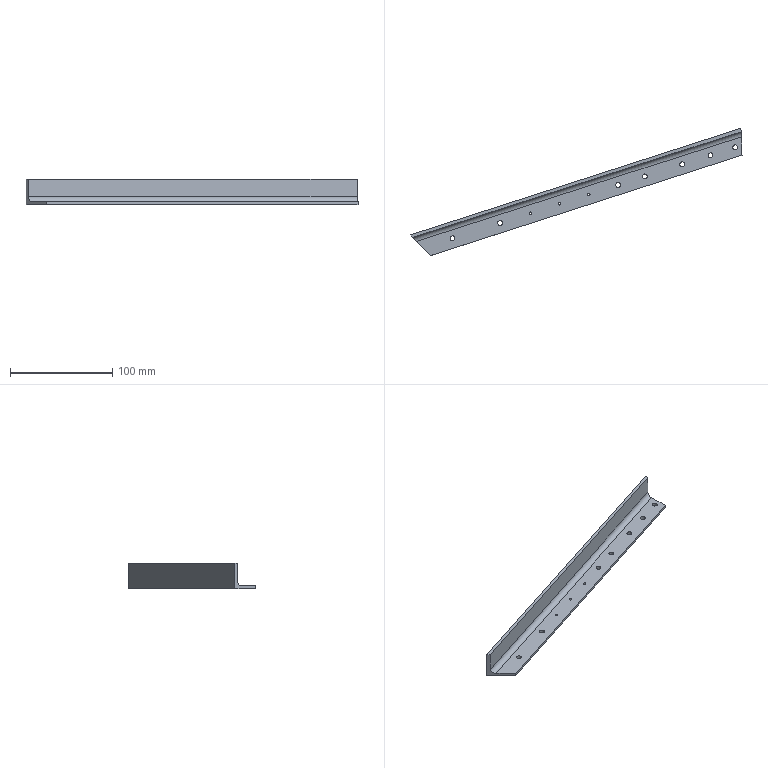Part | NX | features MG0301 nose pivot 24(right) 2 | 1 solid | 19 faces | box 324.725 x 124.459 x 25.4 mm | volume 51732 mm3 | cylinder 11 | plane 8 | commonest cylinder face diameters 4.763 x7 2.4 x3 9.525 x1
STEP:
#1=CARTESIAN_POINT('',(-201.575,-73.399,0.));
#2=VERTEX_POINT('',#1);
#3=CARTESIAN_POINT('',(-202.775,-73.399,0.));
#4=DIRECTION('',(0.,0.,1.));
#5=DIRECTION('',(1.,0.,0.));
#6=AXIS2_PLACEMENT_3D('',#3,#4,#5);
#7=CIRCLE('',#6,1.2);
#8=EDGE_CURVE('',#2,#2,#7,.F.);
#9=ORIENTED_EDGE('',*,*,#8,.F.);
#10=EDGE_LOOP('',(#9));
#11=FACE_BOUND('',#10,.T.);
#12=CARTESIAN_POINT('',(-143.279,-55.017,0.));
#13=VERTEX_POINT('',#12);
#14=CARTESIAN_POINT('',(-145.66,-55.017,0.));
#15=DIRECTION('',(0.,0.,1.));
#16=DIRECTION('',(1.,0.,0.));
#17=AXIS2_PLACEMENT_3D('',#14,#15,#16);
#18=CIRCLE('',#17,2.381);
#19=EDGE_CURVE('',#13,#13,#18,.F.);
#20=ORIENTED_EDGE('',*,*,#19,.F.);
#21=EDGE_LOOP('',(#20));
#22=FACE_BOUND('',#21,.T.);
#23=CARTESIAN_POINT('',(-80.464,-34.801,0.));
#24=VERTEX_POINT('',#23);
#25=CARTESIAN_POINT('',(-82.845,-34.801,0.));
#26=DIRECTION('',(0.,0.,1.));
#27=DIRECTION('',(1.,0.,0.));
#28=AXIS2_PLACEMENT_3D('',#25,#26,#27);
#29=CIRCLE('',#28,2.381);
#30=EDGE_CURVE('',#24,#24,#29,.F.);
#31=ORIENTED_EDGE('',*,*,#30,.F.);
#32=EDGE_LOOP('',(#31));
#33=FACE_BOUND('',#32,.T.);
#34=CARTESIAN_POINT('',(-258.604,-92.134,0.));
#35=VERTEX_POINT('',#34);
#36=CARTESIAN_POINT('',(-260.985,-92.134,0.));
#37=DIRECTION('',(0.,0.,1.));
#38=DIRECTION('',(1.,0.,0.));
#39=AXIS2_PLACEMENT_3D('',#36,#37,#38);
#40=CIRCLE('',#39,2.381);
#41=EDGE_CURVE('',#35,#35,#40,.T.);
#42=ORIENTED_EDGE('',*,*,#41,.T.);
#43=EDGE_LOOP('',(#42));
#44=FACE_BOUND('',#43,.T.);
#45=CARTESIAN_POINT('',(-305.21,-107.134,0.));
#46=VERTEX_POINT('',#45);
#47=CARTESIAN_POINT('',(-307.591,-107.134,0.));
#48=DIRECTION('',(0.,0.,1.));
#49=DIRECTION('',(1.,0.,0.));
#50=AXIS2_PLACEMENT_3D('',#47,#48,#49);
#51=CIRCLE('',#50,2.381);
#52=EDGE_CURVE('',#46,#46,#51,.T.);
#53=ORIENTED_EDGE('',*,*,#52,.T.);
#54=EDGE_LOOP('',(#53));
#55=FACE_BOUND('',#54,.T.);
#56=CARTESIAN_POINT('',(-28.683,-18.135,0.));
#57=VERTEX_POINT('',#56);
#58=CARTESIAN_POINT('',(-31.064,-18.135,0.));
#59=DIRECTION('',(0.,0.,1.));
#60=DIRECTION('',(1.,0.,0.));
#61=AXIS2_PLACEMENT_3D('',#58,#59,#60);
#62=CIRCLE('',#61,2.381);
#63=EDGE_CURVE('',#57,#57,#62,.T.);
#64=ORIENTED_EDGE('',*,*,#63,.T.);
#65=EDGE_LOOP('',(#64));
#66=FACE_BOUND('',#65,.T.);
#67=CARTESIAN_POINT('',(-52.861,-25.917,0.));
#68=VERTEX_POINT('',#67);
#69=CARTESIAN_POINT('',(-55.242,-25.917,0.));
#70=DIRECTION('',(0.,0.,1.));
#71=DIRECTION('',(1.,0.,0.));
#72=AXIS2_PLACEMENT_3D('',#69,#70,#71);
#73=CIRCLE('',#72,2.381);
#74=EDGE_CURVE('',#68,#68,#73,.T.);
#75=ORIENTED_EDGE('',*,*,#74,.T.);
#76=EDGE_LOOP('',(#75));
#77=FACE_BOUND('',#76,.T.);
#78=CARTESIAN_POINT('',(-24.401,-25.997,0.));
#79=VERTEX_POINT('',#78);
#80=CARTESIAN_POINT('',(-329.234,-124.106,0.));
#81=VERTEX_POINT('',#80);
#82=CARTESIAN_POINT('',(-9.84,-21.311,0.));
#83=DIRECTION('',(-0.9519,-0.3064,0.));
#84=VECTOR('',#83,1000.);
#85=LINE('',#82,#84);
#86=EDGE_CURVE('',#79,#81,#85,.T.);
#87=ORIENTED_EDGE('',*,*,#86,.T.);
#88=CARTESIAN_POINT('',(-349.126,-103.825,0.));
#89=VERTEX_POINT('',#88);
#90=CARTESIAN_POINT('',(-239.917,-215.167,0.));
#91=DIRECTION('',(0.7002,-0.7139,0.));
#92=VECTOR('',#91,1000.);
#93=LINE('',#90,#92);
#94=EDGE_CURVE('',#89,#81,#93,.T.);
#95=ORIENTED_EDGE('',*,*,#94,.F.);
#96=CARTESIAN_POINT('',(-25.433,0.3536,0.));
#97=VERTEX_POINT('',#96);
#98=CARTESIAN_POINT('',(-17.622,2.868,0.));
#99=DIRECTION('',(-0.9519,-0.3064,0.));
#100=VECTOR('',#99,1000.);
#101=LINE('',#98,#100);
#102=EDGE_CURVE('',#97,#89,#101,.T.);
#103=ORIENTED_EDGE('',*,*,#102,.F.);
#104=CARTESIAN_POINT('',(-25.52,2.558,0.));
#105=DIRECTION('',(-0.03915,0.9992,0.));
#106=VECTOR('',#105,1000.);
#107=LINE('',#104,#106);
#108=EDGE_CURVE('',#79,#97,#107,.T.);
#109=ORIENTED_EDGE('',*,*,#108,.F.);
#110=EDGE_LOOP('',(#87,#95,#103,#109));
#111=FACE_BOUND('',#110,.T.);
#112=CARTESIAN_POINT('',(-117.106,-46.594,0.));
#113=VERTEX_POINT('',#112);
#114=CARTESIAN_POINT('',(-119.487,-46.594,0.));
#115=DIRECTION('',(0.,0.,1.));
#116=DIRECTION('',(1.,0.,0.));
#117=AXIS2_PLACEMENT_3D('',#114,#115,#116);
#118=CIRCLE('',#117,2.381);
#119=EDGE_CURVE('',#113,#113,#118,.F.);
#120=ORIENTED_EDGE('',*,*,#119,.F.);
#121=EDGE_LOOP('',(#120));
#122=FACE_BOUND('',#121,.T.);
#123=CARTESIAN_POINT('',(-173.017,-64.208,0.));
#124=VERTEX_POINT('',#123);
#125=CARTESIAN_POINT('',(-174.217,-64.208,0.));
#126=DIRECTION('',(0.,0.,1.));
#127=DIRECTION('',(1.,0.,0.));
#128=AXIS2_PLACEMENT_3D('',#125,#126,#127);
#129=CIRCLE('',#128,1.2);
#130=EDGE_CURVE('',#124,#124,#129,.F.);
#131=ORIENTED_EDGE('',*,*,#130,.F.);
#132=EDGE_LOOP('',(#131));
#133=FACE_BOUND('',#132,.T.);
#134=CARTESIAN_POINT('',(-230.132,-82.59,0.));
#135=VERTEX_POINT('',#134);
#136=CARTESIAN_POINT('',(-231.332,-82.59,0.));
#137=DIRECTION('',(0.,0.,1.));
#138=DIRECTION('',(1.,0.,0.));
#139=AXIS2_PLACEMENT_3D('',#136,#137,#138);
#140=CIRCLE('',#139,1.2);
#141=EDGE_CURVE('',#135,#135,#140,.F.);
#142=ORIENTED_EDGE('',*,*,#141,.F.);
#143=EDGE_LOOP('',(#142));
#144=FACE_BOUND('',#143,.T.);
#145=CARTESIAN_POINT('',(-17.622,2.868,0.));
#146=DIRECTION('',(0.,0.,1.));
#147=DIRECTION('',(-1.,0.,0.));
#148=AXIS2_PLACEMENT_3D('',#145,#146,#147);
#149=PLANE('',#148);
#150=ADVANCED_FACE('',(#11,#22,#33,#44,#55,#66,#77,#111,#122,#133,#144),#149,.F.);
#151=CARTESIAN_POINT('',(-202.775,-72.199,3.175));
#152=VERTEX_POINT('',#151);
#153=CARTESIAN_POINT('',(-202.775,-73.399,3.175));
#154=DIRECTION('',(0.,0.,-1.));
#155=DIRECTION('',(0.,1.,0.));
#156=AXIS2_PLACEMENT_3D('',#153,#154,#155);
#157=CIRCLE('',#156,1.2);
#158=EDGE_CURVE('',#152,#152,#157,.F.);
#159=ORIENTED_EDGE('',*,*,#158,.F.);
#160=EDGE_LOOP('',(#159));
#161=FACE_BOUND('',#160,.T.);
#162=CARTESIAN_POINT('',(-145.66,-52.636,3.175));
#163=VERTEX_POINT('',#162);
#164=CARTESIAN_POINT('',(-145.66,-55.017,3.175));
#165=DIRECTION('',(0.,0.,-1.));
#166=DIRECTION('',(0.,1.,0.));
#167=AXIS2_PLACEMENT_3D('',#164,#165,#166);
#168=CIRCLE('',#167,2.381);
#169=EDGE_CURVE('',#163,#163,#168,.T.);
#170=ORIENTED_EDGE('',*,*,#169,.T.);
#171=EDGE_LOOP('',(#170));
#172=FACE_BOUND('',#171,.T.);
#173=CARTESIAN_POINT('',(-82.845,-32.42,3.175));
#174=VERTEX_POINT('',#173);
#175=CARTESIAN_POINT('',(-82.845,-34.801,3.175));
#176=DIRECTION('',(0.,0.,-1.));
#177=DIRECTION('',(0.,1.,0.));
#178=AXIS2_PLACEMENT_3D('',#175,#176,#177);
#179=CIRCLE('',#178,2.381);
#180=EDGE_CURVE('',#174,#174,#179,.T.);
#181=ORIENTED_EDGE('',*,*,#180,.T.);
#182=EDGE_LOOP('',(#181));
#183=FACE_BOUND('',#182,.T.);
#184=CARTESIAN_POINT('',(-260.985,-94.515,3.175));
#185=VERTEX_POINT('',#184);
#186=CARTESIAN_POINT('',(-260.985,-92.134,3.175));
#187=DIRECTION('',(0.,0.,1.));
#188=DIRECTION('',(0.,-1.,0.));
#189=AXIS2_PLACEMENT_3D('',#186,#187,#188);
#190=CIRCLE('',#189,2.381);
#191=EDGE_CURVE('',#185,#185,#190,.T.);
#192=ORIENTED_EDGE('',*,*,#191,.F.);
#193=EDGE_LOOP('',(#192));
#194=FACE_BOUND('',#193,.T.);
#195=CARTESIAN_POINT('',(-307.591,-109.515,3.175));
#196=VERTEX_POINT('',#195);
#197=CARTESIAN_POINT('',(-307.591,-107.134,3.175));
#198=DIRECTION('',(0.,0.,1.));
#199=DIRECTION('',(0.,-1.,0.));
#200=AXIS2_PLACEMENT_3D('',#197,#198,#199);
#201=CIRCLE('',#200,2.381);
#202=EDGE_CURVE('',#196,#196,#201,.T.);
#203=ORIENTED_EDGE('',*,*,#202,.F.);
#204=EDGE_LOOP('',(#203));
#205=FACE_BOUND('',#204,.T.);
#206=CARTESIAN_POINT('',(-31.064,-20.517,3.175));
#207=VERTEX_POINT('',#206);
#208=CARTESIAN_POINT('',(-31.064,-18.135,3.175));
#209=DIRECTION('',(0.,0.,1.));
#210=DIRECTION('',(0.,-1.,0.));
#211=AXIS2_PLACEMENT_3D('',#208,#209,#210);
#212=CIRCLE('',#211,2.381);
#213=EDGE_CURVE('',#207,#207,#212,.T.);
#214=ORIENTED_EDGE('',*,*,#213,.F.);
#215=EDGE_LOOP('',(#214));
#216=FACE_BOUND('',#215,.T.);
#217=CARTESIAN_POINT('',(-55.242,-28.298,3.175));
#218=VERTEX_POINT('',#217);
#219=CARTESIAN_POINT('',(-55.242,-25.917,3.175));
#220=DIRECTION('',(0.,0.,1.));
#221=DIRECTION('',(0.,-1.,0.));
#222=AXIS2_PLACEMENT_3D('',#219,#220,#221);
#223=CIRCLE('',#222,2.381);
#224=EDGE_CURVE('',#218,#218,#223,.T.);
#225=ORIENTED_EDGE('',*,*,#224,.F.);
#226=EDGE_LOOP('',(#225));
#227=FACE_BOUND('',#226,.T.);
#228=CARTESIAN_POINT('',(-25.111,-7.881,3.175));
#229=VERTEX_POINT('',#228);
#230=CARTESIAN_POINT('',(-342.91,-110.162,3.175));
#231=VERTEX_POINT('',#230);
#232=CARTESIAN_POINT('',(-15.19,-4.688,3.175));
#233=DIRECTION('',(-0.9519,-0.3064,0.));
#234=VECTOR('',#233,1000.);
#235=LINE('',#232,#234);
#236=EDGE_CURVE('',#229,#231,#235,.T.);
#237=ORIENTED_EDGE('',*,*,#236,.T.);
#238=CARTESIAN_POINT('',(-329.234,-124.106,3.175));
#239=VERTEX_POINT('',#238);
#240=CARTESIAN_POINT('',(-224.014,-231.381,3.175));
#241=DIRECTION('',(-0.7002,0.7139,0.));
#242=VECTOR('',#241,1000.);
#243=LINE('',#240,#242);
#244=EDGE_CURVE('',#239,#231,#243,.T.);
#245=ORIENTED_EDGE('',*,*,#244,.F.);
#246=CARTESIAN_POINT('',(-24.401,-25.997,3.175));
#247=VERTEX_POINT('',#246);
#248=CARTESIAN_POINT('',(-9.84,-21.311,3.175));
#249=DIRECTION('',(-0.9519,-0.3064,0.));
#250=VECTOR('',#249,1000.);
#251=LINE('',#248,#250);
#252=EDGE_CURVE('',#247,#239,#251,.T.);
#253=ORIENTED_EDGE('',*,*,#252,.F.);
#254=CARTESIAN_POINT('',(-24.562,-21.888,3.175));
#255=DIRECTION('',(0.03915,-0.9992,0.));
#256=VECTOR('',#255,1000.);
#257=LINE('',#254,#256);
#258=EDGE_CURVE('',#229,#247,#257,.T.);
#259=ORIENTED_EDGE('',*,*,#258,.F.);
#260=EDGE_LOOP('',(#237,#245,#253,#259));
#261=FACE_BOUND('',#260,.T.);
#262=CARTESIAN_POINT('',(-119.487,-44.213,3.175));
#263=VERTEX_POINT('',#262);
#264=CARTESIAN_POINT('',(-119.487,-46.594,3.175));
#265=DIRECTION('',(0.,0.,-1.));
#266=DIRECTION('',(0.,1.,0.));
#267=AXIS2_PLACEMENT_3D('',#264,#265,#266);
#268=CIRCLE('',#267,2.381);
#269=EDGE_CURVE('',#263,#263,#268,.T.);
#270=ORIENTED_EDGE('',*,*,#269,.T.);
#271=EDGE_LOOP('',(#270));
#272=FACE_BOUND('',#271,.T.);
#273=CARTESIAN_POINT('',(-174.217,-63.008,3.175));
#274=VERTEX_POINT('',#273);
#275=CARTESIAN_POINT('',(-174.217,-64.208,3.175));
#276=DIRECTION('',(0.,0.,-1.));
#277=DIRECTION('',(0.,1.,0.));
#278=AXIS2_PLACEMENT_3D('',#275,#276,#277);
#279=CIRCLE('',#278,1.2);
#280=EDGE_CURVE('',#274,#274,#279,.F.);
#281=ORIENTED_EDGE('',*,*,#280,.F.);
#282=EDGE_LOOP('',(#281));
#283=FACE_BOUND('',#282,.T.);
#284=CARTESIAN_POINT('',(-231.332,-81.39,3.175));
#285=VERTEX_POINT('',#284);
#286=CARTESIAN_POINT('',(-231.332,-82.59,3.175));
#287=DIRECTION('',(0.,0.,-1.));
#288=DIRECTION('',(0.,1.,0.));
#289=AXIS2_PLACEMENT_3D('',#286,#287,#288);
#290=CIRCLE('',#289,1.2);
#291=EDGE_CURVE('',#285,#285,#290,.F.);
#292=ORIENTED_EDGE('',*,*,#291,.F.);
#293=EDGE_LOOP('',(#292));
#294=FACE_BOUND('',#293,.T.);
#295=CARTESIAN_POINT('',(-9.84,-21.311,3.175));
#296=DIRECTION('',(0.,0.,-1.));
#297=DIRECTION('',(0.,-1.,0.));
#298=AXIS2_PLACEMENT_3D('',#295,#296,#297);
#299=PLANE('',#298);
#300=ADVANCED_FACE('',(#161,#172,#183,#194,#205,#216,#227,#261,#272,#283,#294),#299,.F.);
#301=CARTESIAN_POINT('',(-25.433,0.3536,25.4));
#302=VERTEX_POINT('',#301);
#303=CARTESIAN_POINT('',(-25.433,0.3536,0.));
#304=DIRECTION('',(0.,0.,1.));
#305=VECTOR('',#304,1000.);
#306=LINE('',#303,#305);
#307=EDGE_CURVE('',#97,#302,#306,.T.);
#308=ORIENTED_EDGE('',*,*,#307,.T.);
#309=CARTESIAN_POINT('',(-25.304,-2.94,25.4));
#310=VERTEX_POINT('',#309);
#311=CARTESIAN_POINT('',(-25.52,2.558,25.4));
#312=DIRECTION('',(0.03915,-0.9992,0.));
#313=VECTOR('',#312,1000.);
#314=LINE('',#311,#313);
#315=EDGE_CURVE('',#302,#310,#314,.T.);
#316=ORIENTED_EDGE('',*,*,#315,.T.);
#317=CARTESIAN_POINT('',(-25.304,-2.94,7.938));
#318=VERTEX_POINT('',#317);
#319=CARTESIAN_POINT('',(-25.304,-2.94,25.4));
#320=DIRECTION('',(0.,0.,-1.));
#321=VECTOR('',#320,1000.);
#322=LINE('',#319,#321);
#323=EDGE_CURVE('',#310,#318,#322,.T.);
#324=ORIENTED_EDGE('',*,*,#323,.T.);
#325=CARTESIAN_POINT('',(-25.111,-7.881,7.938));
#326=DIRECTION('',(0.9992,0.03915,0.));
#327=DIRECTION('',(0.03915,-0.9992,0.));
#328=AXIS2_PLACEMENT_3D('',#325,#326,#327);
#329=ELLIPSE('',#328,4.945,4.763);
#330=EDGE_CURVE('',#318,#229,#329,.F.);
#331=ORIENTED_EDGE('',*,*,#330,.T.);
#332=ORIENTED_EDGE('',*,*,#258,.T.);
#333=CARTESIAN_POINT('',(-24.401,-25.997,0.));
#334=DIRECTION('',(0.,0.,-1.));
#335=VECTOR('',#334,1000.);
#336=LINE('',#333,#335);
#337=EDGE_CURVE('',#247,#79,#336,.T.);
#338=ORIENTED_EDGE('',*,*,#337,.T.);
#339=ORIENTED_EDGE('',*,*,#108,.T.);
#340=EDGE_LOOP('',(#308,#316,#324,#331,#332,#338,#339));
#341=FACE_BOUND('',#340,.T.);
#342=CARTESIAN_POINT('',(-26.325,23.115,-842.534));
#343=DIRECTION('',(-0.9992,-0.03915,0.));
#344=DIRECTION('',(0.03915,-0.9992,0.));
#345=AXIS2_PLACEMENT_3D('',#342,#343,#344);
#346=PLANE('',#345);
#347=ADVANCED_FACE('',(#341),#346,.F.);
#348=ORIENTED_EDGE('',*,*,#102,.T.);
#349=CARTESIAN_POINT('',(-349.126,-103.825,25.4));
#350=VERTEX_POINT('',#349);
#351=CARTESIAN_POINT('',(-349.126,-103.825,0.));
#352=DIRECTION('',(0.,0.,-1.));
#353=VECTOR('',#352,1000.);
#354=LINE('',#351,#353);
#355=EDGE_CURVE('',#350,#89,#354,.T.);
#356=ORIENTED_EDGE('',*,*,#355,.F.);
#357=CARTESIAN_POINT('',(-17.622,2.868,25.4));
#358=DIRECTION('',(-0.9519,-0.3064,0.));
#359=VECTOR('',#358,1000.);
#360=LINE('',#357,#359);
#361=EDGE_CURVE('',#302,#350,#360,.T.);
#362=ORIENTED_EDGE('',*,*,#361,.F.);
#363=ORIENTED_EDGE('',*,*,#307,.F.);
#364=EDGE_LOOP('',(#348,#356,#362,#363));
#365=FACE_BOUND('',#364,.T.);
#366=CARTESIAN_POINT('',(-17.622,2.868,0.));
#367=DIRECTION('',(0.3064,-0.9519,0.));
#368=DIRECTION('',(0.9519,0.3064,0.));
#369=AXIS2_PLACEMENT_3D('',#366,#367,#368);
#370=PLANE('',#369);
#371=ADVANCED_FACE('',(#365),#370,.F.);
#372=ORIENTED_EDGE('',*,*,#252,.T.);
#373=CARTESIAN_POINT('',(-329.234,-124.106,0.));
#374=DIRECTION('',(0.,0.,1.));
#375=VECTOR('',#374,1000.);
#376=LINE('',#373,#375);
#377=EDGE_CURVE('',#81,#239,#376,.T.);
#378=ORIENTED_EDGE('',*,*,#377,.F.);
#379=ORIENTED_EDGE('',*,*,#86,.F.);
#380=ORIENTED_EDGE('',*,*,#337,.F.);
#381=EDGE_LOOP('',(#372,#378,#379,#380));
#382=FACE_BOUND('',#381,.T.);
#383=CARTESIAN_POINT('',(-9.84,-21.311,0.));
#384=DIRECTION('',(-0.3064,0.9519,0.));
#385=DIRECTION('',(-0.9519,-0.3064,0.));
#386=AXIS2_PLACEMENT_3D('',#383,#384,#385);
#387=PLANE('',#386);
#388=ADVANCED_FACE('',(#382),#387,.F.);
#389=CARTESIAN_POINT('',(-346.639,-106.36,7.938));
#390=VERTEX_POINT('',#389);
#391=CARTESIAN_POINT('',(-16.649,-0.1548,7.938));
#392=DIRECTION('',(-0.9519,-0.3064,0.));
#393=VECTOR('',#392,1000.);
#394=LINE('',#391,#393);
#395=EDGE_CURVE('',#318,#390,#394,.T.);
#396=ORIENTED_EDGE('',*,*,#395,.T.);
#397=CARTESIAN_POINT('',(-342.91,-110.162,7.938));
#398=DIRECTION('',(-0.7139,-0.7002,0.));
#399=DIRECTION('',(-0.7002,0.7139,0.));
#400=AXIS2_PLACEMENT_3D('',#397,#398,#399);
#401=ELLIPSE('',#400,5.327,4.763);
#402=EDGE_CURVE('',#231,#390,#401,.F.);
#403=ORIENTED_EDGE('',*,*,#402,.F.);
#404=ORIENTED_EDGE('',*,*,#236,.F.);
#405=ORIENTED_EDGE('',*,*,#330,.F.);
#406=EDGE_LOOP('',(#396,#403,#404,#405));
#407=FACE_BOUND('',#406,.T.);
#408=CARTESIAN_POINT('',(-15.19,-4.688,7.938));
#409=DIRECTION('',(-0.9519,-0.3064,0.));
#410=DIRECTION('',(0.3064,-0.9519,0.));
#411=AXIS2_PLACEMENT_3D('',#408,#409,#410);
#412=CYLINDRICAL_SURFACE('',#411,4.763);
#413=ADVANCED_FACE('',(#407),#412,.F.);
#414=CARTESIAN_POINT('',(-346.639,-106.36,25.4));
#415=VERTEX_POINT('',#414);
#416=CARTESIAN_POINT('',(-16.649,-0.1548,25.4));
#417=DIRECTION('',(-0.9519,-0.3064,0.));
#418=VECTOR('',#417,1000.);
#419=LINE('',#416,#418);
#420=EDGE_CURVE('',#310,#415,#419,.T.);
#421=ORIENTED_EDGE('',*,*,#420,.T.);
#422=CARTESIAN_POINT('',(-346.639,-106.36,25.4));
#423=DIRECTION('',(0.,0.,1.));
#424=VECTOR('',#423,1000.);
#425=LINE('',#422,#424);
#426=EDGE_CURVE('',#390,#415,#425,.T.);
#427=ORIENTED_EDGE('',*,*,#426,.F.);
#428=ORIENTED_EDGE('',*,*,#395,.F.);
#429=ORIENTED_EDGE('',*,*,#323,.F.);
#430=EDGE_LOOP('',(#421,#427,#428,#429));
#431=FACE_BOUND('',#430,.T.);
#432=CARTESIAN_POINT('',(-16.649,-0.1548,25.4));
#433=DIRECTION('',(-0.3064,0.9519,0.));
#434=DIRECTION('',(-0.9519,-0.3064,0.));
#435=AXIS2_PLACEMENT_3D('',#432,#433,#434);
#436=PLANE('',#435);
#437=ADVANCED_FACE('',(#431),#436,.F.);
#438=ORIENTED_EDGE('',*,*,#361,.T.);
#439=CARTESIAN_POINT('',(-239.917,-215.167,25.4));
#440=DIRECTION('',(-0.7002,0.7139,0.));
#441=VECTOR('',#440,1000.);
#442=LINE('',#439,#441);
#443=EDGE_CURVE('',#415,#350,#442,.T.);
#444=ORIENTED_EDGE('',*,*,#443,.F.);
#445=ORIENTED_EDGE('',*,*,#420,.F.);
#446=ORIENTED_EDGE('',*,*,#315,.F.);
#447=EDGE_LOOP('',(#438,#444,#445,#446));
#448=FACE_BOUND('',#447,.T.);
#449=CARTESIAN_POINT('',(-17.622,2.868,25.4));
#450=DIRECTION('',(0.,0.,-1.));
#451=DIRECTION('',(1.,0.,0.));
#452=AXIS2_PLACEMENT_3D('',#449,#450,#451);
#453=PLANE('',#452);
#454=ADVANCED_FACE('',(#448),#453,.F.);
#455=ORIENTED_EDGE('',*,*,#355,.T.);
#456=ORIENTED_EDGE('',*,*,#94,.T.);
#457=ORIENTED_EDGE('',*,*,#377,.T.);
#458=ORIENTED_EDGE('',*,*,#244,.T.);
#459=ORIENTED_EDGE('',*,*,#402,.T.);
#460=ORIENTED_EDGE('',*,*,#426,.T.);
#461=ORIENTED_EDGE('',*,*,#443,.T.);
#462=EDGE_LOOP('',(#455,#456,#457,#458,#459,#460,#461));
#463=FACE_BOUND('',#462,.T.);
#464=CARTESIAN_POINT('',(-368.345,-84.23,-842.534));
#465=DIRECTION('',(0.7139,0.7002,0.));
#466=DIRECTION('',(-0.7002,0.7139,0.));
#467=AXIS2_PLACEMENT_3D('',#464,#465,#466);
#468=PLANE('',#467);
#469=ADVANCED_FACE('',(#463),#468,.F.);
#470=ORIENTED_EDGE('',*,*,#74,.F.);
#471=EDGE_LOOP('',(#470));
#472=FACE_BOUND('',#471,.T.);
#473=ORIENTED_EDGE('',*,*,#224,.T.);
#474=EDGE_LOOP('',(#473));
#475=FACE_BOUND('',#474,.T.);
#476=CARTESIAN_POINT('',(-55.242,-25.917,63.5));
#477=DIRECTION('',(0.,0.,-1.));
#478=DIRECTION('',(1.,0.,0.));
#479=AXIS2_PLACEMENT_3D('',#476,#477,#478);
#480=CYLINDRICAL_SURFACE('',#479,2.381);
#481=ADVANCED_FACE('',(#472,#475),#480,.F.);
#482=ORIENTED_EDGE('',*,*,#63,.F.);
#483=EDGE_LOOP('',(#482));
#484=FACE_BOUND('',#483,.T.);
#485=ORIENTED_EDGE('',*,*,#213,.T.);
#486=EDGE_LOOP('',(#485));
#487=FACE_BOUND('',#486,.T.);
#488=CARTESIAN_POINT('',(-31.064,-18.135,63.5));
#489=DIRECTION('',(0.,0.,-1.));
#490=DIRECTION('',(1.,0.,0.));
#491=AXIS2_PLACEMENT_3D('',#488,#489,#490);
#492=CYLINDRICAL_SURFACE('',#491,2.381);
#493=ADVANCED_FACE('',(#484,#487),#492,.F.);
#494=ORIENTED_EDGE('',*,*,#52,.F.);
#495=EDGE_LOOP('',(#494));
#496=FACE_BOUND('',#495,.T.);
#497=ORIENTED_EDGE('',*,*,#202,.T.);
#498=EDGE_LOOP('',(#497));
#499=FACE_BOUND('',#498,.T.);
#500=CARTESIAN_POINT('',(-307.591,-107.134,63.5));
#501=DIRECTION('',(0.,0.,-1.));
#502=DIRECTION('',(1.,0.,0.));
#503=AXIS2_PLACEMENT_3D('',#500,#501,#502);
#504=CYLINDRICAL_SURFACE('',#503,2.381);
#505=ADVANCED_FACE('',(#496,#499),#504,.F.);
#506=ORIENTED_EDGE('',*,*,#41,.F.);
#507=EDGE_LOOP('',(#506));
#508=FACE_BOUND('',#507,.T.);
#509=ORIENTED_EDGE('',*,*,#191,.T.);
#510=EDGE_LOOP('',(#509));
#511=FACE_BOUND('',#510,.T.);
#512=CARTESIAN_POINT('',(-260.985,-92.134,63.5));
#513=DIRECTION('',(0.,0.,-1.));
#514=DIRECTION('',(1.,0.,0.));
#515=AXIS2_PLACEMENT_3D('',#512,#513,#514);
#516=CYLINDRICAL_SURFACE('',#515,2.381);
#517=ADVANCED_FACE('',(#508,#511),#516,.F.);
#518=ORIENTED_EDGE('',*,*,#180,.F.);
#519=EDGE_LOOP('',(#518));
#520=FACE_BOUND('',#519,.T.);
#521=ORIENTED_EDGE('',*,*,#30,.T.);
#522=EDGE_LOOP('',(#521));
#523=FACE_BOUND('',#522,.T.);
#524=CARTESIAN_POINT('',(-82.845,-34.801,4.175));
#525=DIRECTION('',(0.,0.,-1.));
#526=DIRECTION('',(0.,1.,0.));
#527=AXIS2_PLACEMENT_3D('',#524,#525,#526);
#528=CYLINDRICAL_SURFACE('',#527,2.381);
#529=ADVANCED_FACE('',(#520,#523),#528,.F.);
#530=ORIENTED_EDGE('',*,*,#269,.F.);
#531=EDGE_LOOP('',(#530));
#532=FACE_BOUND('',#531,.T.);
#533=ORIENTED_EDGE('',*,*,#119,.T.);
#534=EDGE_LOOP('',(#533));
#535=FACE_BOUND('',#534,.T.);
#536=CARTESIAN_POINT('',(-119.487,-46.594,4.175));
#537=DIRECTION('',(0.,0.,-1.));
#538=DIRECTION('',(0.,1.,0.));
#539=AXIS2_PLACEMENT_3D('',#536,#537,#538);
#540=CYLINDRICAL_SURFACE('',#539,2.381);
#541=ADVANCED_FACE('',(#532,#535),#540,.F.);
#542=ORIENTED_EDGE('',*,*,#169,.F.);
#543=EDGE_LOOP('',(#542));
#544=FACE_BOUND('',#543,.T.);
#545=ORIENTED_EDGE('',*,*,#19,.T.);
#546=EDGE_LOOP('',(#545));
#547=FACE_BOUND('',#546,.T.);
#548=CARTESIAN_POINT('',(-145.66,-55.017,4.175));
#549=DIRECTION('',(0.,0.,-1.));
#550=DIRECTION('',(0.,1.,0.));
#551=AXIS2_PLACEMENT_3D('',#548,#549,#550);
#552=CYLINDRICAL_SURFACE('',#551,2.381);
#553=ADVANCED_FACE('',(#544,#547),#552,.F.);
#554=ORIENTED_EDGE('',*,*,#280,.T.);
#555=EDGE_LOOP('',(#554));
#556=FACE_BOUND('',#555,.T.);
#557=ORIENTED_EDGE('',*,*,#130,.T.);
#558=EDGE_LOOP('',(#557));
#559=FACE_BOUND('',#558,.T.);
#560=CARTESIAN_POINT('',(-174.217,-64.208,4.175));
#561=DIRECTION('',(0.,0.,-1.));
#562=DIRECTION('',(0.,1.,0.));
#563=AXIS2_PLACEMENT_3D('',#560,#561,#562);
#564=CYLINDRICAL_SURFACE('',#563,1.2);
#565=ADVANCED_FACE('',(#556,#559),#564,.F.);
#566=ORIENTED_EDGE('',*,*,#158,.T.);
#567=EDGE_LOOP('',(#566));
#568=FACE_BOUND('',#567,.T.);
#569=ORIENTED_EDGE('',*,*,#8,.T.);
#570=EDGE_LOOP('',(#569));
#571=FACE_BOUND('',#570,.T.);
#572=CARTESIAN_POINT('',(-202.775,-73.399,4.175));
#573=DIRECTION('',(0.,0.,-1.));
#574=DIRECTION('',(0.,1.,0.));
#575=AXIS2_PLACEMENT_3D('',#572,#573,#574);
#576=CYLINDRICAL_SURFACE('',#575,1.2);
#577=ADVANCED_FACE('',(#568,#571),#576,.F.);
#578=ORIENTED_EDGE('',*,*,#291,.T.);
#579=EDGE_LOOP('',(#578));
#580=FACE_BOUND('',#579,.T.);
#581=ORIENTED_EDGE('',*,*,#141,.T.);
#582=EDGE_LOOP('',(#581));
#583=FACE_BOUND('',#582,.T.);
#584=CARTESIAN_POINT('',(-231.332,-82.59,4.175));
#585=DIRECTION('',(0.,0.,-1.));
#586=DIRECTION('',(0.,1.,0.));
#587=AXIS2_PLACEMENT_3D('',#584,#585,#586);
#588=CYLINDRICAL_SURFACE('',#587,1.2);
#589=ADVANCED_FACE('',(#580,#583),#588,.F.);
#590=CLOSED_SHELL('',(#150,#300,#347,#371,#388,#413,#437,#454,#469,#481,#493,#505,#517,#529,#541,#553,#565,#577,#589));
#591=MANIFOLD_SOLID_BREP('',#590);
#592=(LENGTH_UNIT()NAMED_UNIT(*)SI_UNIT(.MILLI.,.METRE.));
#593=UNCERTAINTY_MEASURE_WITH_UNIT(LENGTH_MEASURE(0.00001),#592,'','');
#594=(NAMED_UNIT(*)PLANE_ANGLE_UNIT()SI_UNIT($,.RADIAN.));
#595=(NAMED_UNIT(*)SI_UNIT($,.STERADIAN.)SOLID_ANGLE_UNIT());
#596=(GEOMETRIC_REPRESENTATION_CONTEXT(3)GLOBAL_UNCERTAINTY_ASSIGNED_CONTEXT((#593))GLOBAL_UNIT_ASSIGNED_CONTEXT((#592,#594,#595))REPRESENTATION_CONTEXT('',''));
#597=ADVANCED_BREP_SHAPE_REPRESENTATION('',(#591),#596);